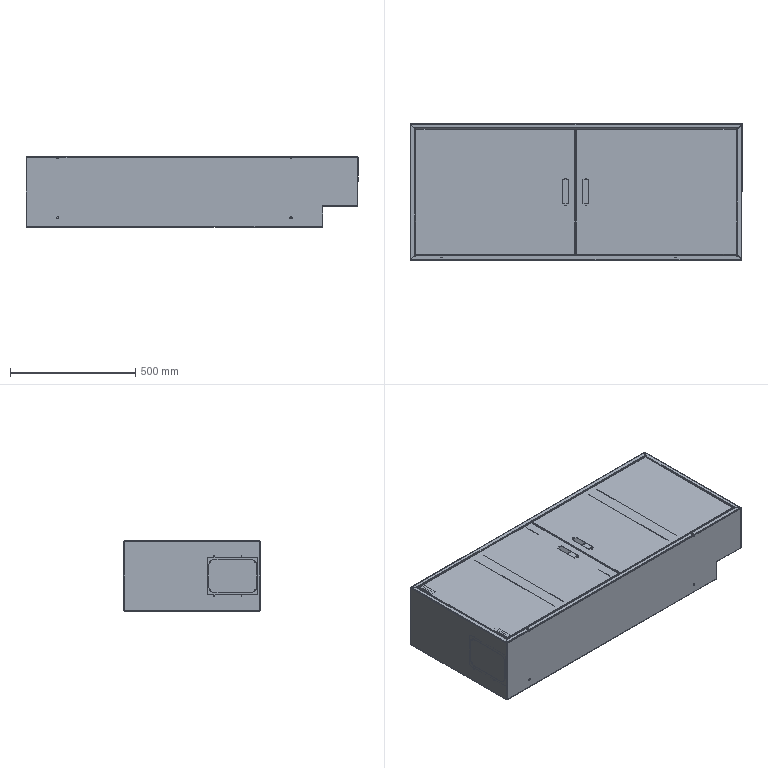Part | SolidWorks | 13 solids | 630 faces | box 1324 x 545 x 280 mm | volume 5513701 mm3 | plane 332 | cylinder 220 | spline 72 | torus 4 | cone 2 | commonest cylinder face diameters 6 x36 1.473 x28 4.473 x28 2 x24 9 x22 3.3 x16